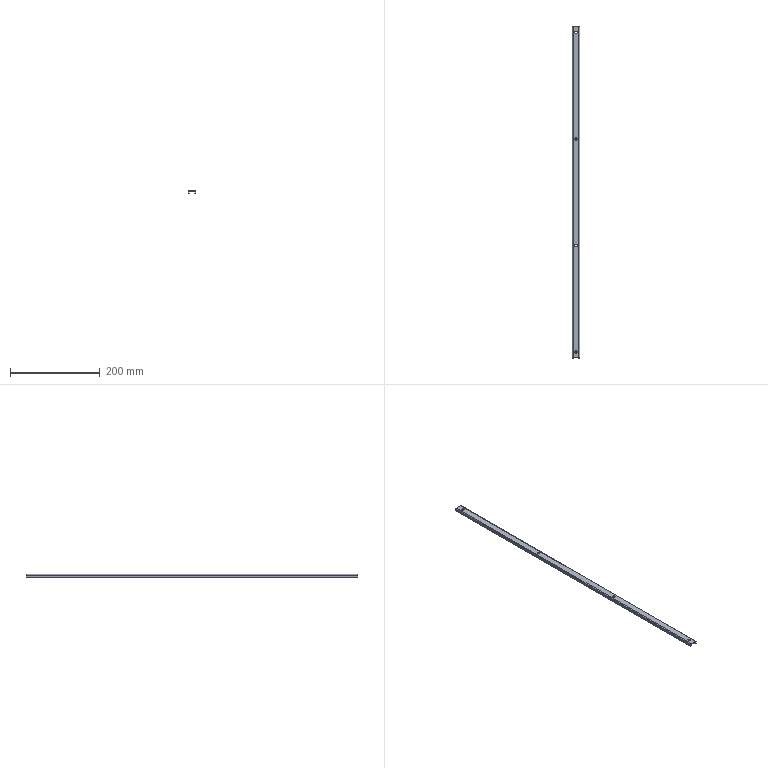Part | NX | features BREP 1 | 1 solid | 40 faces | box 17 x 738 x 7 mm | volume 38096 mm3 | plane 22 | cone 8 | cylinder 6 | torus 4 | commonest cylinder face diameters 0.2 x2 2 x2 4.2 x2
STEP:
#1=CARTESIAN_POINT('',(-2.7,355.,2.));
#2=VERTEX_POINT('',#1);
#3=CARTESIAN_POINT('',(2.7,355.,2.));
#4=VERTEX_POINT('',#3);
#5=CARTESIAN_POINT('',(0.,355.,2.));
#6=DIRECTION('',(0.,0.,1.));
#7=DIRECTION('',(1.,0.,0.));
#8=AXIS2_PLACEMENT_3D('',#5,#6,#7);
#9=CIRCLE('',#8,2.7);
#10=EDGE_CURVE('',#2,#4,#9,.T.);
#11=ORIENTED_EDGE('',*,*,#10,.T.);
#12=CARTESIAN_POINT('',(4.7,355.,0.));
#13=VERTEX_POINT('',#12);
#14=CARTESIAN_POINT('',(4.7,355.,0.));
#15=DIRECTION('',(0.7071,0.,-0.7071));
#16=VECTOR('',#15,1000.);
#17=LINE('',#14,#16);
#18=EDGE_CURVE('',#4,#13,#17,.T.);
#19=ORIENTED_EDGE('',*,*,#18,.T.);
#20=CARTESIAN_POINT('',(-4.7,355.,0.));
#21=VERTEX_POINT('',#20);
#22=CARTESIAN_POINT('',(0.,355.,0.));
#23=DIRECTION('',(0.,0.,-1.));
#24=DIRECTION('',(-1.,0.,0.));
#25=AXIS2_PLACEMENT_3D('',#22,#23,#24);
#26=CIRCLE('',#25,4.7);
#27=EDGE_CURVE('',#13,#21,#26,.T.);
#28=ORIENTED_EDGE('',*,*,#27,.T.);
#29=CARTESIAN_POINT('',(-4.7,355.,0.));
#30=DIRECTION('',(-0.7071,0.,-0.7071));
#31=VECTOR('',#30,1000.);
#32=LINE('',#29,#31);
#33=EDGE_CURVE('',#2,#21,#32,.T.);
#34=ORIENTED_EDGE('',*,*,#33,.F.);
#35=EDGE_LOOP('',(#11,#19,#28,#34));
#36=FACE_BOUND('',#35,.T.);
#37=CARTESIAN_POINT('',(0.,355.,0.));
#38=DIRECTION('',(0.,0.,-1.));
#39=DIRECTION('',(-1.,0.,0.));
#40=AXIS2_PLACEMENT_3D('',#37,#38,#39);
#41=CONICAL_SURFACE('',#40,4.7,0.7854);
#42=ADVANCED_FACE('',(#36),#41,.F.);
#43=CARTESIAN_POINT('',(-2.7,118.,2.));
#44=VERTEX_POINT('',#43);
#45=CARTESIAN_POINT('',(2.7,118.,2.));
#46=VERTEX_POINT('',#45);
#47=CARTESIAN_POINT('',(0.,118.,2.));
#48=DIRECTION('',(0.,0.,1.));
#49=DIRECTION('',(1.,0.,0.));
#50=AXIS2_PLACEMENT_3D('',#47,#48,#49);
#51=CIRCLE('',#50,2.7);
#52=EDGE_CURVE('',#44,#46,#51,.T.);
#53=ORIENTED_EDGE('',*,*,#52,.T.);
#54=CARTESIAN_POINT('',(4.7,118.,0.));
#55=VERTEX_POINT('',#54);
#56=CARTESIAN_POINT('',(4.7,118.,0.));
#57=DIRECTION('',(0.7071,0.,-0.7071));
#58=VECTOR('',#57,1000.);
#59=LINE('',#56,#58);
#60=EDGE_CURVE('',#46,#55,#59,.T.);
#61=ORIENTED_EDGE('',*,*,#60,.T.);
#62=CARTESIAN_POINT('',(-4.7,118.,0.));
#63=VERTEX_POINT('',#62);
#64=CARTESIAN_POINT('',(0.,118.,0.));
#65=DIRECTION('',(0.,0.,-1.));
#66=DIRECTION('',(-1.,0.,0.));
#67=AXIS2_PLACEMENT_3D('',#64,#65,#66);
#68=CIRCLE('',#67,4.7);
#69=EDGE_CURVE('',#55,#63,#68,.T.);
#70=ORIENTED_EDGE('',*,*,#69,.T.);
#71=CARTESIAN_POINT('',(-4.7,118.,0.));
#72=DIRECTION('',(-0.7071,0.,-0.7071));
#73=VECTOR('',#72,1000.);
#74=LINE('',#71,#73);
#75=EDGE_CURVE('',#44,#63,#74,.T.);
#76=ORIENTED_EDGE('',*,*,#75,.F.);
#77=EDGE_LOOP('',(#53,#61,#70,#76));
#78=FACE_BOUND('',#77,.T.);
#79=CARTESIAN_POINT('',(0.,118.,0.));
#80=DIRECTION('',(0.,0.,-1.));
#81=DIRECTION('',(-1.,0.,0.));
#82=AXIS2_PLACEMENT_3D('',#79,#80,#81);
#83=CONICAL_SURFACE('',#82,4.7,0.7854);
#84=ADVANCED_FACE('',(#78),#83,.F.);
#85=CARTESIAN_POINT('',(-2.7,-119.,2.));
#86=VERTEX_POINT('',#85);
#87=CARTESIAN_POINT('',(2.7,-119.,2.));
#88=VERTEX_POINT('',#87);
#89=CARTESIAN_POINT('',(0.,-119.,2.));
#90=DIRECTION('',(0.,0.,1.));
#91=DIRECTION('',(1.,0.,0.));
#92=AXIS2_PLACEMENT_3D('',#89,#90,#91);
#93=CIRCLE('',#92,2.7);
#94=EDGE_CURVE('',#86,#88,#93,.T.);
#95=ORIENTED_EDGE('',*,*,#94,.T.);
#96=CARTESIAN_POINT('',(4.7,-119.,0.));
#97=VERTEX_POINT('',#96);
#98=CARTESIAN_POINT('',(4.7,-119.,0.));
#99=DIRECTION('',(0.7071,0.,-0.7071));
#100=VECTOR('',#99,1000.);
#101=LINE('',#98,#100);
#102=EDGE_CURVE('',#88,#97,#101,.T.);
#103=ORIENTED_EDGE('',*,*,#102,.T.);
#104=CARTESIAN_POINT('',(-4.7,-119.,0.));
#105=VERTEX_POINT('',#104);
#106=CARTESIAN_POINT('',(0.,-119.,0.));
#107=DIRECTION('',(0.,0.,-1.));
#108=DIRECTION('',(-1.,0.,0.));
#109=AXIS2_PLACEMENT_3D('',#106,#107,#108);
#110=CIRCLE('',#109,4.7);
#111=EDGE_CURVE('',#97,#105,#110,.T.);
#112=ORIENTED_EDGE('',*,*,#111,.T.);
#113=CARTESIAN_POINT('',(-4.7,-119.,0.));
#114=DIRECTION('',(-0.7071,0.,-0.7071));
#115=VECTOR('',#114,1000.);
#116=LINE('',#113,#115);
#117=EDGE_CURVE('',#86,#105,#116,.T.);
#118=ORIENTED_EDGE('',*,*,#117,.F.);
#119=EDGE_LOOP('',(#95,#103,#112,#118));
#120=FACE_BOUND('',#119,.T.);
#121=CARTESIAN_POINT('',(0.,-119.,0.));
#122=DIRECTION('',(0.,0.,-1.));
#123=DIRECTION('',(-1.,0.,0.));
#124=AXIS2_PLACEMENT_3D('',#121,#122,#123);
#125=CONICAL_SURFACE('',#124,4.7,0.7854);
#126=ADVANCED_FACE('',(#120),#125,.F.);
#127=CARTESIAN_POINT('',(-2.7,-356.,2.));
#128=VERTEX_POINT('',#127);
#129=CARTESIAN_POINT('',(2.7,-356.,2.));
#130=VERTEX_POINT('',#129);
#131=CARTESIAN_POINT('',(0.,-356.,2.));
#132=DIRECTION('',(0.,0.,1.));
#133=DIRECTION('',(1.,0.,0.));
#134=AXIS2_PLACEMENT_3D('',#131,#132,#133);
#135=CIRCLE('',#134,2.7);
#136=EDGE_CURVE('',#128,#130,#135,.T.);
#137=ORIENTED_EDGE('',*,*,#136,.T.);
#138=CARTESIAN_POINT('',(4.7,-356.,0.));
#139=VERTEX_POINT('',#138);
#140=CARTESIAN_POINT('',(4.7,-356.,0.));
#141=DIRECTION('',(0.7071,0.,-0.7071));
#142=VECTOR('',#141,1000.);
#143=LINE('',#140,#142);
#144=EDGE_CURVE('',#130,#139,#143,.T.);
#145=ORIENTED_EDGE('',*,*,#144,.T.);
#146=CARTESIAN_POINT('',(-4.7,-356.,0.));
#147=VERTEX_POINT('',#146);
#148=CARTESIAN_POINT('',(0.,-356.,0.));
#149=DIRECTION('',(0.,0.,-1.));
#150=DIRECTION('',(-1.,0.,0.));
#151=AXIS2_PLACEMENT_3D('',#148,#149,#150);
#152=CIRCLE('',#151,4.7);
#153=EDGE_CURVE('',#139,#147,#152,.T.);
#154=ORIENTED_EDGE('',*,*,#153,.T.);
#155=CARTESIAN_POINT('',(-4.7,-356.,0.));
#156=DIRECTION('',(-0.7071,0.,-0.7071));
#157=VECTOR('',#156,1000.);
#158=LINE('',#155,#157);
#159=EDGE_CURVE('',#128,#147,#158,.T.);
#160=ORIENTED_EDGE('',*,*,#159,.F.);
#161=EDGE_LOOP('',(#137,#145,#154,#160));
#162=FACE_BOUND('',#161,.T.);
#163=CARTESIAN_POINT('',(0.,-356.,0.));
#164=DIRECTION('',(0.,0.,-1.));
#165=DIRECTION('',(-1.,0.,0.));
#166=AXIS2_PLACEMENT_3D('',#163,#164,#165);
#167=CONICAL_SURFACE('',#166,4.7,0.7854);
#168=ADVANCED_FACE('',(#162),#167,.F.);
#169=CARTESIAN_POINT('',(-6.4,368.,0.));
#170=VERTEX_POINT('',#169);
#171=CARTESIAN_POINT('',(-6.4,-368.,0.));
#172=VERTEX_POINT('',#171);
#173=CARTESIAN_POINT('',(-6.4,369.,0.));
#174=DIRECTION('',(0.,-1.,0.));
#175=VECTOR('',#174,1000.);
#176=LINE('',#173,#175);
#177=EDGE_CURVE('',#170,#172,#176,.T.);
#178=ORIENTED_EDGE('',*,*,#177,.F.);
#179=CARTESIAN_POINT('',(6.4,368.,0.));
#180=VERTEX_POINT('',#179);
#181=CARTESIAN_POINT('',(6.4,368.,0.));
#182=DIRECTION('',(1.,0.,0.));
#183=VECTOR('',#182,1000.);
#184=LINE('',#181,#183);
#185=EDGE_CURVE('',#170,#180,#184,.T.);
#186=ORIENTED_EDGE('',*,*,#185,.T.);
#187=CARTESIAN_POINT('',(6.4,-368.,0.));
#188=VERTEX_POINT('',#187);
#189=CARTESIAN_POINT('',(6.4,369.,0.));
#190=DIRECTION('',(0.,-1.,0.));
#191=VECTOR('',#190,1000.);
#192=LINE('',#189,#191);
#193=EDGE_CURVE('',#180,#188,#192,.T.);
#194=ORIENTED_EDGE('',*,*,#193,.T.);
#195=CARTESIAN_POINT('',(-6.4,-368.,0.));
#196=DIRECTION('',(-1.,0.,0.));
#197=VECTOR('',#196,1000.);
#198=LINE('',#195,#197);
#199=EDGE_CURVE('',#188,#172,#198,.T.);
#200=ORIENTED_EDGE('',*,*,#199,.T.);
#201=EDGE_LOOP('',(#178,#186,#194,#200));
#202=FACE_BOUND('',#201,.T.);
#203=CARTESIAN_POINT('',(0.,355.,0.));
#204=DIRECTION('',(0.,0.,-1.));
#205=DIRECTION('',(-1.,0.,0.));
#206=AXIS2_PLACEMENT_3D('',#203,#204,#205);
#207=CIRCLE('',#206,4.7);
#208=EDGE_CURVE('',#21,#13,#207,.T.);
#209=ORIENTED_EDGE('',*,*,#208,.F.);
#210=ORIENTED_EDGE('',*,*,#27,.F.);
#211=EDGE_LOOP('',(#209,#210));
#212=FACE_BOUND('',#211,.T.);
#213=CARTESIAN_POINT('',(0.,118.,0.));
#214=DIRECTION('',(0.,0.,-1.));
#215=DIRECTION('',(-1.,0.,0.));
#216=AXIS2_PLACEMENT_3D('',#213,#214,#215);
#217=CIRCLE('',#216,4.7);
#218=EDGE_CURVE('',#63,#55,#217,.T.);
#219=ORIENTED_EDGE('',*,*,#218,.F.);
#220=ORIENTED_EDGE('',*,*,#69,.F.);
#221=EDGE_LOOP('',(#219,#220));
#222=FACE_BOUND('',#221,.T.);
#223=CARTESIAN_POINT('',(0.,-356.,0.));
#224=DIRECTION('',(0.,0.,-1.));
#225=DIRECTION('',(-1.,0.,0.));
#226=AXIS2_PLACEMENT_3D('',#223,#224,#225);
#227=CIRCLE('',#226,4.7);
#228=EDGE_CURVE('',#147,#139,#227,.T.);
#229=ORIENTED_EDGE('',*,*,#228,.F.);
#230=ORIENTED_EDGE('',*,*,#153,.F.);
#231=EDGE_LOOP('',(#229,#230));
#232=FACE_BOUND('',#231,.T.);
#233=CARTESIAN_POINT('',(0.,-119.,0.));
#234=DIRECTION('',(0.,0.,-1.));
#235=DIRECTION('',(-1.,0.,0.));
#236=AXIS2_PLACEMENT_3D('',#233,#234,#235);
#237=CIRCLE('',#236,4.7);
#238=EDGE_CURVE('',#105,#97,#237,.T.);
#239=ORIENTED_EDGE('',*,*,#238,.F.);
#240=ORIENTED_EDGE('',*,*,#111,.F.);
#241=EDGE_LOOP('',(#239,#240));
#242=FACE_BOUND('',#241,.T.);
#243=CARTESIAN_POINT('',(-6.5,369.,0.));
#244=DIRECTION('',(0.,0.,1.));
#245=DIRECTION('',(1.,0.,0.));
#246=AXIS2_PLACEMENT_3D('',#243,#244,#245);
#247=PLANE('',#246);
#248=ADVANCED_FACE('',(#202,#212,#222,#232,#242),#247,.F.);
#249=CARTESIAN_POINT('',(6.4,-369.,2.));
#250=VERTEX_POINT('',#249);
#251=CARTESIAN_POINT('',(-6.4,-369.,2.));
#252=VERTEX_POINT('',#251);
#253=CARTESIAN_POINT('',(-6.5,-369.,2.));
#254=DIRECTION('',(-1.,0.,0.));
#255=VECTOR('',#254,1000.);
#256=LINE('',#253,#255);
#257=EDGE_CURVE('',#250,#252,#256,.T.);
#258=ORIENTED_EDGE('',*,*,#257,.F.);
#259=CARTESIAN_POINT('',(6.4,369.,2.));
#260=VERTEX_POINT('',#259);
#261=CARTESIAN_POINT('',(6.4,369.,2.));
#262=DIRECTION('',(0.,-1.,0.));
#263=VECTOR('',#262,1000.);
#264=LINE('',#261,#263);
#265=EDGE_CURVE('',#260,#250,#264,.T.);
#266=ORIENTED_EDGE('',*,*,#265,.F.);
#267=CARTESIAN_POINT('',(-6.4,369.,2.));
#268=VERTEX_POINT('',#267);
#269=CARTESIAN_POINT('',(-6.5,369.,2.));
#270=DIRECTION('',(-1.,0.,0.));
#271=VECTOR('',#270,1000.);
#272=LINE('',#269,#271);
#273=EDGE_CURVE('',#260,#268,#272,.T.);
#274=ORIENTED_EDGE('',*,*,#273,.T.);
#275=CARTESIAN_POINT('',(-6.4,369.,2.));
#276=DIRECTION('',(0.,-1.,0.));
#277=VECTOR('',#276,1000.);
#278=LINE('',#275,#277);
#279=EDGE_CURVE('',#268,#252,#278,.T.);
#280=ORIENTED_EDGE('',*,*,#279,.T.);
#281=EDGE_LOOP('',(#258,#266,#274,#280));
#282=FACE_BOUND('',#281,.T.);
#283=ORIENTED_EDGE('',*,*,#10,.F.);
#284=CARTESIAN_POINT('',(0.,355.,2.));
#285=DIRECTION('',(0.,0.,1.));
#286=DIRECTION('',(1.,0.,0.));
#287=AXIS2_PLACEMENT_3D('',#284,#285,#286);
#288=CIRCLE('',#287,2.7);
#289=EDGE_CURVE('',#4,#2,#288,.T.);
#290=ORIENTED_EDGE('',*,*,#289,.F.);
#291=EDGE_LOOP('',(#283,#290));
#292=FACE_BOUND('',#291,.T.);
#293=ORIENTED_EDGE('',*,*,#52,.F.);
#294=CARTESIAN_POINT('',(0.,118.,2.));
#295=DIRECTION('',(0.,0.,1.));
#296=DIRECTION('',(1.,0.,0.));
#297=AXIS2_PLACEMENT_3D('',#294,#295,#296);
#298=CIRCLE('',#297,2.7);
#299=EDGE_CURVE('',#46,#44,#298,.T.);
#300=ORIENTED_EDGE('',*,*,#299,.F.);
#301=EDGE_LOOP('',(#293,#300));
#302=FACE_BOUND('',#301,.T.);
#303=ORIENTED_EDGE('',*,*,#94,.F.);
#304=CARTESIAN_POINT('',(0.,-119.,2.));
#305=DIRECTION('',(0.,0.,1.));
#306=DIRECTION('',(1.,0.,0.));
#307=AXIS2_PLACEMENT_3D('',#304,#305,#306);
#308=CIRCLE('',#307,2.7);
#309=EDGE_CURVE('',#88,#86,#308,.T.);
#310=ORIENTED_EDGE('',*,*,#309,.F.);
#311=EDGE_LOOP('',(#303,#310));
#312=FACE_BOUND('',#311,.T.);
#313=ORIENTED_EDGE('',*,*,#136,.F.);
#314=CARTESIAN_POINT('',(0.,-356.,2.));
#315=DIRECTION('',(0.,0.,1.));
#316=DIRECTION('',(1.,0.,0.));
#317=AXIS2_PLACEMENT_3D('',#314,#315,#316);
#318=CIRCLE('',#317,2.7);
#319=EDGE_CURVE('',#130,#128,#318,.T.);
#320=ORIENTED_EDGE('',*,*,#319,.F.);
#321=EDGE_LOOP('',(#313,#320));
#322=FACE_BOUND('',#321,.T.);
#323=CARTESIAN_POINT('',(-6.5,369.,2.));
#324=DIRECTION('',(0.,0.,1.));
#325=DIRECTION('',(1.,0.,0.));
#326=AXIS2_PLACEMENT_3D('',#323,#324,#325);
#327=PLANE('',#326);
#328=ADVANCED_FACE('',(#282,#292,#302,#312,#322),#327,.T.);
#329=CARTESIAN_POINT('',(7.5,369.,-0.1));
#330=VERTEX_POINT('',#329);
#331=CARTESIAN_POINT('',(8.5,369.,-0.1));
#332=VERTEX_POINT('',#331);
#333=CARTESIAN_POINT('',(6.5,369.,-0.1));
#334=DIRECTION('',(1.,0.,0.));
#335=VECTOR('',#334,1000.);
#336=LINE('',#333,#335);
#337=EDGE_CURVE('',#330,#332,#336,.T.);
#338=ORIENTED_EDGE('',*,*,#337,.F.);
#339=CARTESIAN_POINT('',(6.4,369.,1.));
#340=VERTEX_POINT('',#339);
#341=CARTESIAN_POINT('',(6.4,369.,-0.1));
#342=DIRECTION('',(0.,-1.,0.));
#343=DIRECTION('',(0.,0.,1.));
#344=AXIS2_PLACEMENT_3D('',#341,#342,#343);
#345=CIRCLE('',#344,1.1);
#346=EDGE_CURVE('',#330,#340,#345,.T.);
#347=ORIENTED_EDGE('',*,*,#346,.T.);
#348=CARTESIAN_POINT('',(6.4,369.,2.));
#349=DIRECTION('',(0.,0.,-1.));
#350=VECTOR('',#349,1000.);
#351=LINE('',#348,#350);
#352=EDGE_CURVE('',#260,#340,#351,.T.);
#353=ORIENTED_EDGE('',*,*,#352,.F.);
#354=CARTESIAN_POINT('',(6.4,369.,-0.1));
#355=DIRECTION('',(0.,-1.,0.));
#356=DIRECTION('',(1.,0.,0.));
#357=AXIS2_PLACEMENT_3D('',#354,#355,#356);
#358=CIRCLE('',#357,2.1);
#359=EDGE_CURVE('',#332,#260,#358,.T.);
#360=ORIENTED_EDGE('',*,*,#359,.F.);
#361=EDGE_LOOP('',(#338,#347,#353,#360));
#362=FACE_BOUND('',#361,.T.);
#363=CARTESIAN_POINT('',(6.5,369.,-0.1));
#364=DIRECTION('',(0.,1.,0.));
#365=DIRECTION('',(1.,0.,0.));
#366=AXIS2_PLACEMENT_3D('',#363,#364,#365);
#367=PLANE('',#366);
#368=ADVANCED_FACE('',(#362),#367,.T.);
#369=CARTESIAN_POINT('',(8.5,369.,-4.));
#370=VERTEX_POINT('',#369);
#371=CARTESIAN_POINT('',(8.5,369.,0.));
#372=DIRECTION('',(0.,0.,1.));
#373=VECTOR('',#372,1000.);
#374=LINE('',#371,#373);
#375=EDGE_CURVE('',#370,#332,#374,.T.);
#376=ORIENTED_EDGE('',*,*,#375,.F.);
#377=CARTESIAN_POINT('',(6.5,369.,-4.));
#378=VERTEX_POINT('',#377);
#379=CARTESIAN_POINT('',(6.4,369.,-4.));
#380=DIRECTION('',(-1.,0.,0.));
#381=VECTOR('',#380,1000.);
#382=LINE('',#379,#381);
#383=EDGE_CURVE('',#370,#378,#382,.T.);
#384=ORIENTED_EDGE('',*,*,#383,.T.);
#385=CARTESIAN_POINT('',(6.5,369.,-1.195));
#386=VERTEX_POINT('',#385);
#387=CARTESIAN_POINT('',(6.5,369.,0.));
#388=DIRECTION('',(0.,0.,1.));
#389=VECTOR('',#388,1000.);
#390=LINE('',#387,#389);
#391=EDGE_CURVE('',#378,#386,#390,.T.);
#392=ORIENTED_EDGE('',*,*,#391,.T.);
#393=CARTESIAN_POINT('',(6.4,369.,-0.1));
#394=DIRECTION('',(0.,-1.,0.));
#395=DIRECTION('',(0.,0.,1.));
#396=AXIS2_PLACEMENT_3D('',#393,#394,#395);
#397=CIRCLE('',#396,1.1);
#398=EDGE_CURVE('',#386,#330,#397,.T.);
#399=ORIENTED_EDGE('',*,*,#398,.T.);
#400=ORIENTED_EDGE('',*,*,#337,.T.);
#401=EDGE_LOOP('',(#376,#384,#392,#399,#400));
#402=FACE_BOUND('',#401,.T.);
#403=CARTESIAN_POINT('',(6.4,369.,2.));
#404=DIRECTION('',(0.,1.,0.));
#405=DIRECTION('',(1.,0.,0.));
#406=AXIS2_PLACEMENT_3D('',#403,#404,#405);
#407=PLANE('',#406);
#408=ADVANCED_FACE('',(#402),#407,.T.);
#409=CARTESIAN_POINT('',(6.4,-369.,1.));
#410=VERTEX_POINT('',#409);
#411=CARTESIAN_POINT('',(6.4,-369.,0.));
#412=DIRECTION('',(0.,0.,1.));
#413=VECTOR('',#412,1000.);
#414=LINE('',#411,#413);
#415=EDGE_CURVE('',#410,#250,#414,.T.);
#416=ORIENTED_EDGE('',*,*,#415,.F.);
#417=CARTESIAN_POINT('',(7.5,-369.,-0.1));
#418=VERTEX_POINT('',#417);
#419=CARTESIAN_POINT('',(6.4,-369.,-0.1));
#420=DIRECTION('',(0.,1.,0.));
#421=DIRECTION('',(0.,0.,-1.));
#422=AXIS2_PLACEMENT_3D('',#419,#420,#421);
#423=CIRCLE('',#422,1.1);
#424=EDGE_CURVE('',#410,#418,#423,.T.);
#425=ORIENTED_EDGE('',*,*,#424,.T.);
#426=CARTESIAN_POINT('',(8.5,-369.,-0.1));
#427=VERTEX_POINT('',#426);
#428=CARTESIAN_POINT('',(8.5,-369.,-0.1));
#429=DIRECTION('',(-1.,0.,0.));
#430=VECTOR('',#429,1000.);
#431=LINE('',#428,#430);
#432=EDGE_CURVE('',#427,#418,#431,.T.);
#433=ORIENTED_EDGE('',*,*,#432,.F.);
#434=CARTESIAN_POINT('',(6.4,-369.,-0.1));
#435=DIRECTION('',(0.,-1.,0.));
#436=DIRECTION('',(1.,0.,0.));
#437=AXIS2_PLACEMENT_3D('',#434,#435,#436);
#438=CIRCLE('',#437,2.1);
#439=EDGE_CURVE('',#427,#250,#438,.T.);
#440=ORIENTED_EDGE('',*,*,#439,.T.);
#441=EDGE_LOOP('',(#416,#425,#433,#440));
#442=FACE_BOUND('',#441,.T.);
#443=CARTESIAN_POINT('',(6.4,-369.,0.));
#444=DIRECTION('',(0.,-1.,0.));
#445=DIRECTION('',(0.,0.,-1.));
#446=AXIS2_PLACEMENT_3D('',#443,#444,#445);
#447=PLANE('',#446);
#448=ADVANCED_FACE('',(#442),#447,.T.);
#449=CARTESIAN_POINT('',(-6.4,-369.,1.));
#450=VERTEX_POINT('',#449);
#451=CARTESIAN_POINT('',(-6.4,-369.,2.));
#452=DIRECTION('',(0.,0.,-1.));
#453=VECTOR('',#452,1000.);
#454=LINE('',#451,#453);
#455=EDGE_CURVE('',#252,#450,#454,.T.);
#456=ORIENTED_EDGE('',*,*,#455,.T.);
#457=CARTESIAN_POINT('',(6.4,-369.,1.));
#458=DIRECTION('',(1.,0.,0.));
#459=VECTOR('',#458,1000.);
#460=LINE('',#457,#459);
#461=EDGE_CURVE('',#450,#410,#460,.T.);
#462=ORIENTED_EDGE('',*,*,#461,.T.);
#463=ORIENTED_EDGE('',*,*,#415,.T.);
#464=ORIENTED_EDGE('',*,*,#257,.T.);
#465=EDGE_LOOP('',(#456,#462,#463,#464));
#466=FACE_BOUND('',#465,.T.);
#467=CARTESIAN_POINT('',(8.5,-369.,-0.1));
#468=DIRECTION('',(0.,-1.,0.));
#469=DIRECTION('',(0.,0.,-1.));
#470=AXIS2_PLACEMENT_3D('',#467,#468,#469);
#471=PLANE('',#470);
#472=ADVANCED_FACE('',(#466),#471,.T.);
#473=CARTESIAN_POINT('',(-6.4,369.,1.));
#474=VERTEX_POINT('',#473);
#475=CARTESIAN_POINT('',(-6.4,369.,0.));
#476=DIRECTION('',(0.,0.,1.));
#477=VECTOR('',#476,1000.);
#478=LINE('',#475,#477);
#479=EDGE_CURVE('',#474,#268,#478,.T.);
#480=ORIENTED_EDGE('',*,*,#479,.F.);
#481=CARTESIAN_POINT('',(-7.5,369.,-0.1));
#482=VERTEX_POINT('',#481);
#483=CARTESIAN_POINT('',(-6.4,369.,-0.1));
#484=DIRECTION('',(0.,-1.,0.));
#485=DIRECTION('',(0.,0.,1.));
#486=AXIS2_PLACEMENT_3D('',#483,#484,#485);
#487=CIRCLE('',#486,1.1);
#488=EDGE_CURVE('',#474,#482,#487,.T.);
#489=ORIENTED_EDGE('',*,*,#488,.T.);
#490=CARTESIAN_POINT('',(-8.5,369.,-0.1));
#491=VERTEX_POINT('',#490);
#492=CARTESIAN_POINT('',(-8.5,369.,-0.1));
#493=DIRECTION('',(1.,0.,0.));
#494=VECTOR('',#493,1000.);
#495=LINE('',#492,#494);
#496=EDGE_CURVE('',#491,#482,#495,.T.);
#497=ORIENTED_EDGE('',*,*,#496,.F.);
#498=CARTESIAN_POINT('',(-6.4,369.,-0.1));
#499=DIRECTION('',(0.,-1.,0.));
#500=DIRECTION('',(1.,0.,0.));
#501=AXIS2_PLACEMENT_3D('',#498,#499,#500);
#502=CIRCLE('',#501,2.1);
#503=EDGE_CURVE('',#268,#491,#502,.T.);
#504=ORIENTED_EDGE('',*,*,#503,.F.);
#505=EDGE_LOOP('',(#480,#489,#497,#504));
#506=FACE_BOUND('',#505,.T.);
#507=CARTESIAN_POINT('',(-6.4,369.,0.));
#508=DIRECTION('',(0.,1.,0.));
#509=DIRECTION('',(1.,0.,0.));
#510=AXIS2_PLACEMENT_3D('',#507,#508,#509);
#511=PLANE('',#510);
#512=ADVANCED_FACE('',(#506),#511,.T.);
#513=ORIENTED_EDGE('',*,*,#352,.T.);
#514=CARTESIAN_POINT('',(-6.4,369.,1.));
#515=DIRECTION('',(-1.,0.,0.));
#516=VECTOR('',#515,1000.);
#517=LINE('',#514,#516);
#518=EDGE_CURVE('',#340,#474,#517,.T.);
#519=ORIENTED_EDGE('',*,*,#518,.T.);
#520=ORIENTED_EDGE('',*,*,#479,.T.);
#521=ORIENTED_EDGE('',*,*,#273,.F.);
#522=EDGE_LOOP('',(#513,#519,#520,#521));
#523=FACE_BOUND('',#522,.T.);
#524=CARTESIAN_POINT('',(-8.5,369.,-0.1));
#525=DIRECTION('',(0.,1.,0.));
#526=DIRECTION('',(1.,0.,0.));
#527=AXIS2_PLACEMENT_3D('',#524,#525,#526);
#528=PLANE('',#527);
#529=ADVANCED_FACE('',(#523),#528,.T.);
#530=CARTESIAN_POINT('',(-7.5,-369.,-0.1));
#531=VERTEX_POINT('',#530);
#532=CARTESIAN_POINT('',(-8.5,-369.,-0.1));
#533=VERTEX_POINT('',#532);
#534=CARTESIAN_POINT('',(-6.5,-369.,-0.1));
#535=DIRECTION('',(-1.,0.,0.));
#536=VECTOR('',#535,1000.);
#537=LINE('',#534,#536);
#538=EDGE_CURVE('',#531,#533,#537,.T.);
#539=ORIENTED_EDGE('',*,*,#538,.F.);
#540=CARTESIAN_POINT('',(-6.4,-369.,-0.1));
#541=DIRECTION('',(0.,1.,0.));
#542=DIRECTION('',(0.,0.,-1.));
#543=AXIS2_PLACEMENT_3D('',#540,#541,#542);
#544=CIRCLE('',#543,1.1);
#545=EDGE_CURVE('',#531,#450,#544,.T.);
#546=ORIENTED_EDGE('',*,*,#545,.T.);
#547=ORIENTED_EDGE('',*,*,#455,.F.);
#548=CARTESIAN_POINT('',(-6.4,-369.,-0.1));
#549=DIRECTION('',(0.,-1.,0.));
#550=DIRECTION('',(1.,0.,0.));
#551=AXIS2_PLACEMENT_3D('',#548,#549,#550);
#552=CIRCLE('',#551,2.1);
#553=EDGE_CURVE('',#252,#533,#552,.T.);
#554=ORIENTED_EDGE('',*,*,#553,.T.);
#555=EDGE_LOOP('',(#539,#546,#547,#554));
#556=FACE_BOUND('',#555,.T.);
#557=CARTESIAN_POINT('',(-6.5,-369.,-0.1));
#558=DIRECTION('',(0.,-1.,0.));
#559=DIRECTION('',(0.,0.,-1.));
#560=AXIS2_PLACEMENT_3D('',#557,#558,#559);
#561=PLANE('',#560);
#562=ADVANCED_FACE('',(#556),#561,.T.);
#563=CARTESIAN_POINT('',(-8.5,-369.,-4.));
#564=VERTEX_POINT('',#563);
#565=CARTESIAN_POINT('',(-8.5,-369.,0.));
#566=DIRECTION('',(0.,0.,-1.));
#567=VECTOR('',#566,1000.);
#568=LINE('',#565,#567);
#569=EDGE_CURVE('',#533,#564,#568,.T.);
#570=ORIENTED_EDGE('',*,*,#569,.T.);
#571=CARTESIAN_POINT('',(-6.5,-369.,-4.));
#572=VERTEX_POINT('',#571);
#573=CARTESIAN_POINT('',(-6.4,-369.,-4.));
#574=DIRECTION('',(1.,0.,0.));
#575=VECTOR('',#574,1000.);
#576=LINE('',#573,#575);
#577=EDGE_CURVE('',#564,#572,#576,.T.);
#578=ORIENTED_EDGE('',*,*,#577,.T.);
#579=CARTESIAN_POINT('',(-6.5,-369.,-1.195));
#580=VERTEX_POINT('',#579);
#581=CARTESIAN_POINT('',(-6.5,-369.,0.));
#582=DIRECTION('',(0.,0.,-1.));
#583=VECTOR('',#582,1000.);
#584=LINE('',#581,#583);
#585=EDGE_CURVE('',#580,#572,#584,.T.);
#586=ORIENTED_EDGE('',*,*,#585,.F.);
#587=CARTESIAN_POINT('',(-6.4,-369.,-0.1));
#588=DIRECTION('',(0.,1.,0.));
#589=DIRECTION('',(0.,0.,-1.));
#590=AXIS2_PLACEMENT_3D('',#587,#588,#589);
#591=CIRCLE('',#590,1.1);
#592=EDGE_CURVE('',#580,#531,#591,.T.);
#593=ORIENTED_EDGE('',*,*,#592,.T.);
#594=ORIENTED_EDGE('',*,*,#538,.T.);
#595=EDGE_LOOP('',(#570,#578,#586,#593,#594));
#596=FACE_BOUND('',#595,.T.);
#597=CARTESIAN_POINT('',(-6.4,-369.,2.));
#598=DIRECTION('',(0.,-1.,0.));
#599=DIRECTION('',(0.,0.,-1.));
#600=AXIS2_PLACEMENT_3D('',#597,#598,#599);
#601=PLANE('',#600);
#602=ADVANCED_FACE('',(#596),#601,.T.);
#603=CARTESIAN_POINT('',(-6.5,368.,-5.));
#604=VERTEX_POINT('',#603);
#605=CARTESIAN_POINT('',(-6.5,-368.,-5.));
#606=VERTEX_POINT('',#605);
#607=CARTESIAN_POINT('',(-6.5,369.,-5.));
#608=DIRECTION('',(0.,-1.,0.));
#609=VECTOR('',#608,1000.);
#610=LINE('',#607,#609);
#611=EDGE_CURVE('',#604,#606,#610,.T.);
#612=ORIENTED_EDGE('',*,*,#611,.F.);
#613=CARTESIAN_POINT('',(-6.5,369.,-4.));
#614=VERTEX_POINT('',#613);
#615=CARTESIAN_POINT('',(-6.5,368.,-5.));
#616=DIRECTION('',(0.,0.7071,0.7071));
#617=VECTOR('',#616,1000.);
#618=LINE('',#615,#617);
#619=EDGE_CURVE('',#604,#614,#618,.T.);
#620=ORIENTED_EDGE('',*,*,#619,.T.);
#621=CARTESIAN_POINT('',(-6.5,369.,-1.195));
#622=VERTEX_POINT('',#621);
#623=CARTESIAN_POINT('',(-6.5,369.,0.));
#624=DIRECTION('',(0.,0.,-1.));
#625=VECTOR('',#624,1000.);
#626=LINE('',#623,#625);
#627=EDGE_CURVE('',#622,#614,#626,.T.);
#628=ORIENTED_EDGE('',*,*,#627,.F.);
#629=CARTESIAN_POINT('',(-6.5,368.,-0.1));
#630=VERTEX_POINT('',#629);
#631=CARTESIAN_POINT('',(-6.5,369.,-1.195));
#632=CARTESIAN_POINT('',(-6.5,369.,-0.9262));
#633=CARTESIAN_POINT('',(-6.5,368.841,-0.5362));
#634=CARTESIAN_POINT('',(-6.5,368.369,-0.219));
#635=CARTESIAN_POINT('',(-6.5,368.163,-0.1517));
#636=CARTESIAN_POINT('',(-6.5,368.,-0.1));
#637=B_SPLINE_CURVE_WITH_KNOTS('',3,(#631,#632,#633,#634,#635,#636),.UNSPECIFIED.,.F.,.F.,(4,1,1,4),(0.,0.5,0.75,1.),.UNSPECIFIED.);
#638=EDGE_CURVE('',#622,#630,#637,.T.);
#639=ORIENTED_EDGE('',*,*,#638,.T.);
#640=CARTESIAN_POINT('',(-6.5,-368.,-0.1));
#641=VERTEX_POINT('',#640);
#642=CARTESIAN_POINT('',(-6.5,369.,-0.1));
#643=DIRECTION('',(0.,-1.,0.));
#644=VECTOR('',#643,1000.);
#645=LINE('',#642,#644);
#646=EDGE_CURVE('',#630,#641,#645,.T.);
#647=ORIENTED_EDGE('',*,*,#646,.T.);
#648=CARTESIAN_POINT('',(-6.5,-368.,-0.1));
#649=CARTESIAN_POINT('',(-6.5,-368.162,-0.1513));
#650=CARTESIAN_POINT('',(-6.5,-368.369,-0.2191));
#651=CARTESIAN_POINT('',(-6.5,-368.84,-0.5364));
#652=CARTESIAN_POINT('',(-6.5,-369.,-0.9248));
#653=CARTESIAN_POINT('',(-6.5,-369.,-1.195));
#654=B_SPLINE_CURVE_WITH_KNOTS('',3,(#648,#649,#650,#651,#652,#653),.UNSPECIFIED.,.F.,.F.,(4,1,1,4),(0.,0.25,0.5,1.),.UNSPECIFIED.);
#655=EDGE_CURVE('',#641,#580,#654,.T.);
#656=ORIENTED_EDGE('',*,*,#655,.T.);
#657=ORIENTED_EDGE('',*,*,#585,.T.);
#658=CARTESIAN_POINT('',(-6.5,-369.,-4.));
#659=DIRECTION('',(0.,0.7071,-0.7071));
#660=VECTOR('',#659,1000.);
#661=LINE('',#658,#660);
#662=EDGE_CURVE('',#572,#606,#661,.T.);
#663=ORIENTED_EDGE('',*,*,#662,.T.);
#664=EDGE_LOOP('',(#612,#620,#628,#639,#647,#656,#657,#663));
#665=FACE_BOUND('',#664,.T.);
#666=CARTESIAN_POINT('',(-6.5,369.,0.));
#667=DIRECTION('',(-1.,0.,0.));
#668=DIRECTION('',(0.,1.,0.));
#669=AXIS2_PLACEMENT_3D('',#666,#667,#668);
#670=PLANE('',#669);
#671=ADVANCED_FACE('',(#665),#670,.F.);
#672=CARTESIAN_POINT('',(-8.5,368.,-5.));
#673=VERTEX_POINT('',#672);
#674=CARTESIAN_POINT('',(-8.5,-368.,-5.));
#675=VERTEX_POINT('',#674);
#676=CARTESIAN_POINT('',(-8.5,369.,-5.));
#677=DIRECTION('',(0.,-1.,0.));
#678=VECTOR('',#677,1000.);
#679=LINE('',#676,#678);
#680=EDGE_CURVE('',#673,#675,#679,.T.);
#681=ORIENTED_EDGE('',*,*,#680,.F.);
#682=CARTESIAN_POINT('',(-8.5,368.,-5.));
#683=DIRECTION('',(1.,0.,0.));
#684=VECTOR('',#683,1000.);
#685=LINE('',#682,#684);
#686=EDGE_CURVE('',#673,#604,#685,.T.);
#687=ORIENTED_EDGE('',*,*,#686,.T.);
#688=ORIENTED_EDGE('',*,*,#611,.T.);
#689=CARTESIAN_POINT('',(-8.5,-368.,-5.));
#690=DIRECTION('',(-1.,0.,0.));
#691=VECTOR('',#690,1000.);
#692=LINE('',#689,#691);
#693=EDGE_CURVE('',#606,#675,#692,.T.);
#694=ORIENTED_EDGE('',*,*,#693,.T.);
#695=EDGE_LOOP('',(#681,#687,#688,#694));
#696=FACE_BOUND('',#695,.T.);
#697=CARTESIAN_POINT('',(-8.5,369.,-5.));
#698=DIRECTION('',(0.,0.,-1.));
#699=DIRECTION('',(-1.,0.,0.));
#700=AXIS2_PLACEMENT_3D('',#697,#698,#699);
#701=PLANE('',#700);
#702=ADVANCED_FACE('',(#696),#701,.T.);
#703=CARTESIAN_POINT('',(-8.5,369.,-4.));
#704=VERTEX_POINT('',#703);
#705=CARTESIAN_POINT('',(-8.5,369.,0.));
#706=DIRECTION('',(0.,0.,-1.));
#707=VECTOR('',#706,1000.);
#708=LINE('',#705,#707);
#709=EDGE_CURVE('',#491,#704,#708,.T.);
#710=ORIENTED_EDGE('',*,*,#709,.T.);
#711=CARTESIAN_POINT('',(-8.5,371.,-2.));
#712=DIRECTION('',(0.,-0.7071,-0.7071));
#713=VECTOR('',#712,1000.);
#714=LINE('',#711,#713);
#715=EDGE_CURVE('',#704,#673,#714,.T.);
#716=ORIENTED_EDGE('',*,*,#715,.T.);
#717=ORIENTED_EDGE('',*,*,#680,.T.);
#718=CARTESIAN_POINT('',(-8.5,-2.,-371.));
#719=DIRECTION('',(0.,-0.7071,0.7071));
#720=VECTOR('',#719,1000.);
#721=LINE('',#718,#720);
#722=EDGE_CURVE('',#675,#564,#721,.T.);
#723=ORIENTED_EDGE('',*,*,#722,.T.);
#724=ORIENTED_EDGE('',*,*,#569,.F.);
#725=CARTESIAN_POINT('',(-8.5,369.,-0.1));
#726=DIRECTION('',(0.,-1.,0.));
#727=VECTOR('',#726,1000.);
#728=LINE('',#725,#727);
#729=EDGE_CURVE('',#491,#533,#728,.T.);
#730=ORIENTED_EDGE('',*,*,#729,.F.);
#731=EDGE_LOOP('',(#710,#716,#717,#723,#724,#730));
#732=FACE_BOUND('',#731,.T.);
#733=CARTESIAN_POINT('',(-8.5,369.,0.));
#734=DIRECTION('',(-1.,0.,0.));
#735=DIRECTION('',(0.,1.,0.));
#736=AXIS2_PLACEMENT_3D('',#733,#734,#735);
#737=PLANE('',#736);
#738=ADVANCED_FACE('',(#732),#737,.T.);
#739=ORIENTED_EDGE('',*,*,#553,.F.);
#740=ORIENTED_EDGE('',*,*,#279,.F.);
#741=ORIENTED_EDGE('',*,*,#503,.T.);
#742=ORIENTED_EDGE('',*,*,#729,.T.);
#743=EDGE_LOOP('',(#739,#740,#741,#742));
#744=FACE_BOUND('',#743,.T.);
#745=CARTESIAN_POINT('',(-6.4,369.,-0.1));
#746=DIRECTION('',(0.,-1.,0.));
#747=DIRECTION('',(0.,0.,-1.));
#748=AXIS2_PLACEMENT_3D('',#745,#746,#747);
#749=CYLINDRICAL_SURFACE('',#748,2.1);
#750=ADVANCED_FACE('',(#744),#749,.T.);
#751=ORIENTED_EDGE('',*,*,#439,.F.);
#752=CARTESIAN_POINT('',(8.5,369.,-0.1));
#753=DIRECTION('',(0.,-1.,0.));
#754=VECTOR('',#753,1000.);
#755=LINE('',#752,#754);
#756=EDGE_CURVE('',#332,#427,#755,.T.);
#757=ORIENTED_EDGE('',*,*,#756,.F.);
#758=ORIENTED_EDGE('',*,*,#359,.T.);
#759=ORIENTED_EDGE('',*,*,#265,.T.);
#760=EDGE_LOOP('',(#751,#757,#758,#759));
#761=FACE_BOUND('',#760,.T.);
#762=CARTESIAN_POINT('',(6.4,369.,-0.1));
#763=DIRECTION('',(0.,-1.,0.));
#764=DIRECTION('',(0.,0.,-1.));
#765=AXIS2_PLACEMENT_3D('',#762,#763,#764);
#766=CYLINDRICAL_SURFACE('',#765,2.1);
#767=ADVANCED_FACE('',(#761),#766,.T.);
#768=CARTESIAN_POINT('',(8.5,368.,-5.));
#769=VERTEX_POINT('',#768);
#770=CARTESIAN_POINT('',(8.5,-368.,-5.));
#771=VERTEX_POINT('',#770);
#772=CARTESIAN_POINT('',(8.5,369.,-5.));
#773=DIRECTION('',(0.,-1.,0.));
#774=VECTOR('',#773,1000.);
#775=LINE('',#772,#774);
#776=EDGE_CURVE('',#769,#771,#775,.T.);
#777=ORIENTED_EDGE('',*,*,#776,.F.);
#778=CARTESIAN_POINT('',(8.5,371.,-2.));
#779=DIRECTION('',(0.,0.7071,0.7071));
#780=VECTOR('',#779,1000.);
#781=LINE('',#778,#780);
#782=EDGE_CURVE('',#769,#370,#781,.T.);
#783=ORIENTED_EDGE('',*,*,#782,.T.);
#784=ORIENTED_EDGE('',*,*,#375,.T.);
#785=ORIENTED_EDGE('',*,*,#756,.T.);
#786=CARTESIAN_POINT('',(8.5,-369.,-4.));
#787=VERTEX_POINT('',#786);
#788=CARTESIAN_POINT('',(8.5,-369.,0.));
#789=DIRECTION('',(0.,0.,1.));
#790=VECTOR('',#789,1000.);
#791=LINE('',#788,#790);
#792=EDGE_CURVE('',#787,#427,#791,.T.);
#793=ORIENTED_EDGE('',*,*,#792,.F.);
#794=CARTESIAN_POINT('',(8.5,-2.,-371.));
#795=DIRECTION('',(0.,0.7071,-0.7071));
#796=VECTOR('',#795,1000.);
#797=LINE('',#794,#796);
#798=EDGE_CURVE('',#787,#771,#797,.T.);
#799=ORIENTED_EDGE('',*,*,#798,.T.);
#800=EDGE_LOOP('',(#777,#783,#784,#785,#793,#799));
#801=FACE_BOUND('',#800,.T.);
#802=CARTESIAN_POINT('',(8.5,369.,0.));
#803=DIRECTION('',(1.,0.,0.));
#804=DIRECTION('',(0.,1.,0.));
#805=AXIS2_PLACEMENT_3D('',#802,#803,#804);
#806=PLANE('',#805);
#807=ADVANCED_FACE('',(#801),#806,.T.);
#808=CARTESIAN_POINT('',(6.5,368.,-5.));
#809=VERTEX_POINT('',#808);
#810=CARTESIAN_POINT('',(6.5,-368.,-5.));
#811=VERTEX_POINT('',#810);
#812=CARTESIAN_POINT('',(6.5,369.,-5.));
#813=DIRECTION('',(0.,-1.,0.));
#814=VECTOR('',#813,1000.);
#815=LINE('',#812,#814);
#816=EDGE_CURVE('',#809,#811,#815,.T.);
#817=ORIENTED_EDGE('',*,*,#816,.F.);
#818=CARTESIAN_POINT('',(6.5,368.,-5.));
#819=DIRECTION('',(1.,0.,0.));
#820=VECTOR('',#819,1000.);
#821=LINE('',#818,#820);
#822=EDGE_CURVE('',#809,#769,#821,.T.);
#823=ORIENTED_EDGE('',*,*,#822,.T.);
#824=ORIENTED_EDGE('',*,*,#776,.T.);
#825=CARTESIAN_POINT('',(6.5,-368.,-5.));
#826=DIRECTION('',(-1.,0.,0.));
#827=VECTOR('',#826,1000.);
#828=LINE('',#825,#827);
#829=EDGE_CURVE('',#771,#811,#828,.T.);
#830=ORIENTED_EDGE('',*,*,#829,.T.);
#831=EDGE_LOOP('',(#817,#823,#824,#830));
#832=FACE_BOUND('',#831,.T.);
#833=CARTESIAN_POINT('',(6.5,369.,-5.));
#834=DIRECTION('',(0.,0.,-1.));
#835=DIRECTION('',(0.,-1.,0.));
#836=AXIS2_PLACEMENT_3D('',#833,#834,#835);
#837=PLANE('',#836);
#838=ADVANCED_FACE('',(#832),#837,.T.);
#839=ORIENTED_EDGE('',*,*,#391,.F.);
#840=CARTESIAN_POINT('',(6.5,368.,-5.));
#841=DIRECTION('',(0.,-0.7071,-0.7071));
#842=VECTOR('',#841,1000.);
#843=LINE('',#840,#842);
#844=EDGE_CURVE('',#378,#809,#843,.T.);
#845=ORIENTED_EDGE('',*,*,#844,.T.);
#846=ORIENTED_EDGE('',*,*,#816,.T.);
#847=CARTESIAN_POINT('',(6.5,-369.,-4.));
#848=VERTEX_POINT('',#847);
#849=CARTESIAN_POINT('',(6.5,-369.,-4.));
#850=DIRECTION('',(0.,-0.7071,0.7071));
#851=VECTOR('',#850,1000.);
#852=LINE('',#849,#851);
#853=EDGE_CURVE('',#811,#848,#852,.T.);
#854=ORIENTED_EDGE('',*,*,#853,.T.);
#855=CARTESIAN_POINT('',(6.5,-369.,-1.195));
#856=VERTEX_POINT('',#855);
#857=CARTESIAN_POINT('',(6.5,-369.,0.));
#858=DIRECTION('',(0.,0.,1.));
#859=VECTOR('',#858,1000.);
#860=LINE('',#857,#859);
#861=EDGE_CURVE('',#848,#856,#860,.T.);
#862=ORIENTED_EDGE('',*,*,#861,.T.);
#863=CARTESIAN_POINT('',(6.5,-368.,-0.1));
#864=VERTEX_POINT('',#863);
#865=CARTESIAN_POINT('',(6.5,-369.,-1.195));
#866=CARTESIAN_POINT('',(6.5,-369.,-0.9262));
#867=CARTESIAN_POINT('',(6.5,-368.841,-0.5362));
#868=CARTESIAN_POINT('',(6.5,-368.369,-0.219));
#869=CARTESIAN_POINT('',(6.5,-368.163,-0.1517));
#870=CARTESIAN_POINT('',(6.5,-368.,-0.1));
#871=B_SPLINE_CURVE_WITH_KNOTS('',3,(#865,#866,#867,#868,#869,#870),.UNSPECIFIED.,.F.,.F.,(4,1,1,4),(0.,0.5,0.75,1.),.UNSPECIFIED.);
#872=EDGE_CURVE('',#856,#864,#871,.T.);
#873=ORIENTED_EDGE('',*,*,#872,.T.);
#874=CARTESIAN_POINT('',(6.5,368.,-0.1));
#875=VERTEX_POINT('',#874);
#876=CARTESIAN_POINT('',(6.5,369.,-0.1));
#877=DIRECTION('',(0.,-1.,0.));
#878=VECTOR('',#877,1000.);
#879=LINE('',#876,#878);
#880=EDGE_CURVE('',#875,#864,#879,.T.);
#881=ORIENTED_EDGE('',*,*,#880,.F.);
#882=CARTESIAN_POINT('',(6.5,368.,-0.1));
#883=CARTESIAN_POINT('',(6.5,368.162,-0.1513));
#884=CARTESIAN_POINT('',(6.5,368.369,-0.2191));
#885=CARTESIAN_POINT('',(6.5,368.84,-0.5364));
#886=CARTESIAN_POINT('',(6.5,369.,-0.9248));
#887=CARTESIAN_POINT('',(6.5,369.,-1.195));
#888=B_SPLINE_CURVE_WITH_KNOTS('',3,(#882,#883,#884,#885,#886,#887),.UNSPECIFIED.,.F.,.F.,(4,1,1,4),(0.,0.25,0.5,1.),.UNSPECIFIED.);
#889=EDGE_CURVE('',#875,#386,#888,.T.);
#890=ORIENTED_EDGE('',*,*,#889,.T.);
#891=EDGE_LOOP('',(#839,#845,#846,#854,#862,#873,#881,#890));
#892=FACE_BOUND('',#891,.T.);
#893=CARTESIAN_POINT('',(6.5,369.,0.));
#894=DIRECTION('',(1.,0.,0.));
#895=DIRECTION('',(0.,1.,0.));
#896=AXIS2_PLACEMENT_3D('',#893,#894,#895);
#897=PLANE('',#896);
#898=ADVANCED_FACE('',(#892),#897,.F.);
#899=ORIENTED_EDGE('',*,*,#193,.F.);
#900=CARTESIAN_POINT('',(6.4,368.,-0.1));
#901=DIRECTION('',(0.,1.,0.));
#902=DIRECTION('',(0.,0.,1.));
#903=AXIS2_PLACEMENT_3D('',#900,#901,#902);
#904=CIRCLE('',#903,0.1);
#905=EDGE_CURVE('',#180,#875,#904,.T.);
#906=ORIENTED_EDGE('',*,*,#905,.T.);
#907=ORIENTED_EDGE('',*,*,#880,.T.);
#908=CARTESIAN_POINT('',(6.4,-368.,-0.1));
#909=DIRECTION('',(0.,-1.,0.));
#910=DIRECTION('',(0.,0.,-1.));
#911=AXIS2_PLACEMENT_3D('',#908,#909,#910);
#912=CIRCLE('',#911,0.1);
#913=EDGE_CURVE('',#864,#188,#912,.T.);
#914=ORIENTED_EDGE('',*,*,#913,.T.);
#915=EDGE_LOOP('',(#899,#906,#907,#914));
#916=FACE_BOUND('',#915,.T.);
#917=CARTESIAN_POINT('',(6.4,369.,-0.1));
#918=DIRECTION('',(0.,-1.,0.));
#919=DIRECTION('',(0.,0.,-1.));
#920=AXIS2_PLACEMENT_3D('',#917,#918,#919);
#921=CYLINDRICAL_SURFACE('',#920,0.1);
#922=ADVANCED_FACE('',(#916),#921,.F.);
#923=ORIENTED_EDGE('',*,*,#646,.F.);
#924=CARTESIAN_POINT('',(-6.4,368.,-0.1));
#925=DIRECTION('',(0.,1.,0.));
#926=DIRECTION('',(0.,0.,1.));
#927=AXIS2_PLACEMENT_3D('',#924,#925,#926);
#928=CIRCLE('',#927,0.1);
#929=EDGE_CURVE('',#630,#170,#928,.T.);
#930=ORIENTED_EDGE('',*,*,#929,.T.);
#931=ORIENTED_EDGE('',*,*,#177,.T.);
#932=CARTESIAN_POINT('',(-6.4,-368.,-0.1));
#933=DIRECTION('',(0.,-1.,0.));
#934=DIRECTION('',(0.,0.,-1.));
#935=AXIS2_PLACEMENT_3D('',#932,#933,#934);
#936=CIRCLE('',#935,0.1);
#937=EDGE_CURVE('',#172,#641,#936,.T.);
#938=ORIENTED_EDGE('',*,*,#937,.T.);
#939=EDGE_LOOP('',(#923,#930,#931,#938));
#940=FACE_BOUND('',#939,.T.);
#941=CARTESIAN_POINT('',(-6.4,369.,-0.1));
#942=DIRECTION('',(0.,-1.,0.));
#943=DIRECTION('',(0.,0.,-1.));
#944=AXIS2_PLACEMENT_3D('',#941,#942,#943);
#945=CYLINDRICAL_SURFACE('',#944,0.1);
#946=ADVANCED_FACE('',(#940),#945,.F.);
#947=ORIENTED_EDGE('',*,*,#627,.T.);
#948=CARTESIAN_POINT('',(-6.4,369.,-4.));
#949=DIRECTION('',(-1.,0.,0.));
#950=VECTOR('',#949,1000.);
#951=LINE('',#948,#950);
#952=EDGE_CURVE('',#614,#704,#951,.T.);
#953=ORIENTED_EDGE('',*,*,#952,.T.);
#954=ORIENTED_EDGE('',*,*,#709,.F.);
#955=ORIENTED_EDGE('',*,*,#496,.T.);
#956=CARTESIAN_POINT('',(-6.4,369.,-0.1));
#957=DIRECTION('',(0.,-1.,0.));
#958=DIRECTION('',(0.,0.,1.));
#959=AXIS2_PLACEMENT_3D('',#956,#957,#958);
#960=CIRCLE('',#959,1.1);
#961=EDGE_CURVE('',#482,#622,#960,.T.);
#962=ORIENTED_EDGE('',*,*,#961,.T.);
#963=EDGE_LOOP('',(#947,#953,#954,#955,#962));
#964=FACE_BOUND('',#963,.T.);
#965=CARTESIAN_POINT('',(-6.4,369.,-0.1));
#966=DIRECTION('',(0.,1.,0.));
#967=DIRECTION('',(1.,0.,0.));
#968=AXIS2_PLACEMENT_3D('',#965,#966,#967);
#969=PLANE('',#968);
#970=ADVANCED_FACE('',(#964),#969,.T.);
#971=ORIENTED_EDGE('',*,*,#861,.F.);
#972=CARTESIAN_POINT('',(8.5,-369.,-4.));
#973=DIRECTION('',(1.,0.,0.));
#974=VECTOR('',#973,1000.);
#975=LINE('',#972,#974);
#976=EDGE_CURVE('',#848,#787,#975,.T.);
#977=ORIENTED_EDGE('',*,*,#976,.T.);
#978=ORIENTED_EDGE('',*,*,#792,.T.);
#979=ORIENTED_EDGE('',*,*,#432,.T.);
#980=CARTESIAN_POINT('',(6.4,-369.,-0.1));
#981=DIRECTION('',(0.,1.,0.));
#982=DIRECTION('',(0.,0.,-1.));
#983=AXIS2_PLACEMENT_3D('',#980,#981,#982);
#984=CIRCLE('',#983,1.1);
#985=EDGE_CURVE('',#418,#856,#984,.T.);
#986=ORIENTED_EDGE('',*,*,#985,.T.);
#987=EDGE_LOOP('',(#971,#977,#978,#979,#986));
#988=FACE_BOUND('',#987,.T.);
#989=CARTESIAN_POINT('',(-6.4,-369.,-0.1));
#990=DIRECTION('',(0.,1.,0.));
#991=DIRECTION('',(1.,0.,0.));
#992=AXIS2_PLACEMENT_3D('',#989,#990,#991);
#993=PLANE('',#992);
#994=ADVANCED_FACE('',(#988),#993,.F.);
#995=ORIENTED_EDGE('',*,*,#144,.F.);
#996=ORIENTED_EDGE('',*,*,#319,.T.);
#997=ORIENTED_EDGE('',*,*,#159,.T.);
#998=ORIENTED_EDGE('',*,*,#228,.T.);
#999=EDGE_LOOP('',(#995,#996,#997,#998));
#1000=FACE_BOUND('',#999,.T.);
#1001=CARTESIAN_POINT('',(0.,-356.,0.));
#1002=DIRECTION('',(0.,0.,-1.));
#1003=DIRECTION('',(-1.,0.,0.));
#1004=AXIS2_PLACEMENT_3D('',#1001,#1002,#1003);
#1005=CONICAL_SURFACE('',#1004,4.7,0.7854);
#1006=ADVANCED_FACE('',(#1000),#1005,.F.);
#1007=ORIENTED_EDGE('',*,*,#102,.F.);
#1008=ORIENTED_EDGE('',*,*,#309,.T.);
#1009=ORIENTED_EDGE('',*,*,#117,.T.);
#1010=ORIENTED_EDGE('',*,*,#238,.T.);
#1011=EDGE_LOOP('',(#1007,#1008,#1009,#1010));
#1012=FACE_BOUND('',#1011,.T.);
#1013=CARTESIAN_POINT('',(0.,-119.,0.));
#1014=DIRECTION('',(0.,0.,-1.));
#1015=DIRECTION('',(-1.,0.,0.));
#1016=AXIS2_PLACEMENT_3D('',#1013,#1014,#1015);
#1017=CONICAL_SURFACE('',#1016,4.7,0.7854);
#1018=ADVANCED_FACE('',(#1012),#1017,.F.);
#1019=ORIENTED_EDGE('',*,*,#60,.F.);
#1020=ORIENTED_EDGE('',*,*,#299,.T.);
#1021=ORIENTED_EDGE('',*,*,#75,.T.);
#1022=ORIENTED_EDGE('',*,*,#218,.T.);
#1023=EDGE_LOOP('',(#1019,#1020,#1021,#1022));
#1024=FACE_BOUND('',#1023,.T.);
#1025=CARTESIAN_POINT('',(0.,118.,0.));
#1026=DIRECTION('',(0.,0.,-1.));
#1027=DIRECTION('',(-1.,0.,0.));
#1028=AXIS2_PLACEMENT_3D('',#1025,#1026,#1027);
#1029=CONICAL_SURFACE('',#1028,4.7,0.7854);
#1030=ADVANCED_FACE('',(#1024),#1029,.F.);
#1031=ORIENTED_EDGE('',*,*,#18,.F.);
#1032=ORIENTED_EDGE('',*,*,#289,.T.);
#1033=ORIENTED_EDGE('',*,*,#33,.T.);
#1034=ORIENTED_EDGE('',*,*,#208,.T.);
#1035=EDGE_LOOP('',(#1031,#1032,#1033,#1034));
#1036=FACE_BOUND('',#1035,.T.);
#1037=CARTESIAN_POINT('',(0.,355.,0.));
#1038=DIRECTION('',(0.,0.,-1.));
#1039=DIRECTION('',(-1.,0.,0.));
#1040=AXIS2_PLACEMENT_3D('',#1037,#1038,#1039);
#1041=CONICAL_SURFACE('',#1040,4.7,0.7854);
#1042=ADVANCED_FACE('',(#1036),#1041,.F.);
#1043=ORIENTED_EDGE('',*,*,#961,.F.);
#1044=ORIENTED_EDGE('',*,*,#488,.F.);
#1045=CARTESIAN_POINT('',(-6.4,368.,1.));
#1046=DIRECTION('',(1.,0.,0.));
#1047=DIRECTION('',(0.,0.,-1.));
#1048=AXIS2_PLACEMENT_3D('',#1045,#1046,#1047);
#1049=CIRCLE('',#1048,1.);
#1050=EDGE_CURVE('',#170,#474,#1049,.T.);
#1051=ORIENTED_EDGE('',*,*,#1050,.F.);
#1052=ORIENTED_EDGE('',*,*,#929,.F.);
#1053=ORIENTED_EDGE('',*,*,#638,.F.);
#1054=EDGE_LOOP('',(#1043,#1044,#1051,#1052,#1053));
#1055=FACE_BOUND('',#1054,.T.);
#1056=CARTESIAN_POINT('',(-6.4,368.,-0.1));
#1057=DIRECTION('',(0.,1.,0.));
#1058=DIRECTION('',(0.,0.,1.));
#1059=AXIS2_PLACEMENT_3D('',#1056,#1057,#1058);
#1060=TOROIDAL_SURFACE('',#1059,1.1,1.);
#1061=ADVANCED_FACE('',(#1055),#1060,.T.);
#1062=ORIENTED_EDGE('',*,*,#1050,.T.);
#1063=ORIENTED_EDGE('',*,*,#518,.F.);
#1064=CARTESIAN_POINT('',(6.4,368.,1.));
#1065=DIRECTION('',(1.,0.,0.));
#1066=DIRECTION('',(0.,0.,-1.));
#1067=AXIS2_PLACEMENT_3D('',#1064,#1065,#1066);
#1068=CIRCLE('',#1067,1.);
#1069=EDGE_CURVE('',#180,#340,#1068,.T.);
#1070=ORIENTED_EDGE('',*,*,#1069,.F.);
#1071=ORIENTED_EDGE('',*,*,#185,.F.);
#1072=EDGE_LOOP('',(#1062,#1063,#1070,#1071));
#1073=FACE_BOUND('',#1072,.T.);
#1074=CARTESIAN_POINT('',(-8.5,368.,1.));
#1075=DIRECTION('',(1.,0.,0.));
#1076=DIRECTION('',(0.,0.,-1.));
#1077=AXIS2_PLACEMENT_3D('',#1074,#1075,#1076);
#1078=CYLINDRICAL_SURFACE('',#1077,1.);
#1079=ADVANCED_FACE('',(#1073),#1078,.T.);
#1080=ORIENTED_EDGE('',*,*,#889,.F.);
#1081=ORIENTED_EDGE('',*,*,#905,.F.);
#1082=ORIENTED_EDGE('',*,*,#1069,.T.);
#1083=ORIENTED_EDGE('',*,*,#346,.F.);
#1084=ORIENTED_EDGE('',*,*,#398,.F.);
#1085=EDGE_LOOP('',(#1080,#1081,#1082,#1083,#1084));
#1086=FACE_BOUND('',#1085,.T.);
#1087=CARTESIAN_POINT('',(6.4,368.,-0.1));
#1088=DIRECTION('',(0.,1.,0.));
#1089=DIRECTION('',(0.,0.,1.));
#1090=AXIS2_PLACEMENT_3D('',#1087,#1088,#1089);
#1091=TOROIDAL_SURFACE('',#1090,1.1,1.);
#1092=ADVANCED_FACE('',(#1086),#1091,.T.);
#1093=ORIENTED_EDGE('',*,*,#655,.F.);
#1094=ORIENTED_EDGE('',*,*,#937,.F.);
#1095=CARTESIAN_POINT('',(-6.4,-368.,1.));
#1096=DIRECTION('',(1.,0.,0.));
#1097=DIRECTION('',(0.,0.,-1.));
#1098=AXIS2_PLACEMENT_3D('',#1095,#1096,#1097);
#1099=CIRCLE('',#1098,1.);
#1100=EDGE_CURVE('',#450,#172,#1099,.T.);
#1101=ORIENTED_EDGE('',*,*,#1100,.F.);
#1102=ORIENTED_EDGE('',*,*,#545,.F.);
#1103=ORIENTED_EDGE('',*,*,#592,.F.);
#1104=EDGE_LOOP('',(#1093,#1094,#1101,#1102,#1103));
#1105=FACE_BOUND('',#1104,.T.);
#1106=CARTESIAN_POINT('',(-6.4,-368.,-0.1));
#1107=DIRECTION('',(0.,-1.,0.));
#1108=DIRECTION('',(0.,0.,-1.));
#1109=AXIS2_PLACEMENT_3D('',#1106,#1107,#1108);
#1110=TOROIDAL_SURFACE('',#1109,1.1,1.);
#1111=ADVANCED_FACE('',(#1105),#1110,.T.);
#1112=ORIENTED_EDGE('',*,*,#1100,.T.);
#1113=ORIENTED_EDGE('',*,*,#199,.F.);
#1114=CARTESIAN_POINT('',(6.4,-368.,1.));
#1115=DIRECTION('',(1.,0.,0.));
#1116=DIRECTION('',(0.,0.,-1.));
#1117=AXIS2_PLACEMENT_3D('',#1114,#1115,#1116);
#1118=CIRCLE('',#1117,1.);
#1119=EDGE_CURVE('',#410,#188,#1118,.T.);
#1120=ORIENTED_EDGE('',*,*,#1119,.F.);
#1121=ORIENTED_EDGE('',*,*,#461,.F.);
#1122=EDGE_LOOP('',(#1112,#1113,#1120,#1121));
#1123=FACE_BOUND('',#1122,.T.);
#1124=CARTESIAN_POINT('',(-6.5,-368.,1.));
#1125=DIRECTION('',(1.,0.,0.));
#1126=DIRECTION('',(0.,0.,-1.));
#1127=AXIS2_PLACEMENT_3D('',#1124,#1125,#1126);
#1128=CYLINDRICAL_SURFACE('',#1127,1.);
#1129=ADVANCED_FACE('',(#1123),#1128,.T.);
#1130=ORIENTED_EDGE('',*,*,#985,.F.);
#1131=ORIENTED_EDGE('',*,*,#424,.F.);
#1132=ORIENTED_EDGE('',*,*,#1119,.T.);
#1133=ORIENTED_EDGE('',*,*,#913,.F.);
#1134=ORIENTED_EDGE('',*,*,#872,.F.);
#1135=EDGE_LOOP('',(#1130,#1131,#1132,#1133,#1134));
#1136=FACE_BOUND('',#1135,.T.);
#1137=CARTESIAN_POINT('',(6.4,-368.,-0.1));
#1138=DIRECTION('',(0.,-1.,0.));
#1139=DIRECTION('',(0.,0.,-1.));
#1140=AXIS2_PLACEMENT_3D('',#1137,#1138,#1139);
#1141=TOROIDAL_SURFACE('',#1140,1.1,1.);
#1142=ADVANCED_FACE('',(#1136),#1141,.T.);
#1143=ORIENTED_EDGE('',*,*,#715,.F.);
#1144=ORIENTED_EDGE('',*,*,#952,.F.);
#1145=ORIENTED_EDGE('',*,*,#619,.F.);
#1146=ORIENTED_EDGE('',*,*,#686,.F.);
#1147=EDGE_LOOP('',(#1143,#1144,#1145,#1146));
#1148=FACE_BOUND('',#1147,.T.);
#1149=CARTESIAN_POINT('',(-8.5,368.,-5.));
#1150=DIRECTION('',(0.,-0.7071,0.7071));
#1151=DIRECTION('',(-1.,0.,0.));
#1152=AXIS2_PLACEMENT_3D('',#1149,#1150,#1151);
#1153=PLANE('',#1152);
#1154=ADVANCED_FACE('',(#1148),#1153,.F.);
#1155=ORIENTED_EDGE('',*,*,#844,.F.);
#1156=ORIENTED_EDGE('',*,*,#383,.F.);
#1157=ORIENTED_EDGE('',*,*,#782,.F.);
#1158=ORIENTED_EDGE('',*,*,#822,.F.);
#1159=EDGE_LOOP('',(#1155,#1156,#1157,#1158));
#1160=FACE_BOUND('',#1159,.T.);
#1161=CARTESIAN_POINT('',(6.5,368.,-5.));
#1162=DIRECTION('',(0.,-0.7071,0.7071));
#1163=DIRECTION('',(-1.,0.,0.));
#1164=AXIS2_PLACEMENT_3D('',#1161,#1162,#1163);
#1165=PLANE('',#1164);
#1166=ADVANCED_FACE('',(#1160),#1165,.F.);
#1167=ORIENTED_EDGE('',*,*,#853,.F.);
#1168=ORIENTED_EDGE('',*,*,#829,.F.);
#1169=ORIENTED_EDGE('',*,*,#798,.F.);
#1170=ORIENTED_EDGE('',*,*,#976,.F.);
#1171=EDGE_LOOP('',(#1167,#1168,#1169,#1170));
#1172=FACE_BOUND('',#1171,.T.);
#1173=CARTESIAN_POINT('',(-6.4,-369.,-4.));
#1174=DIRECTION('',(0.,-0.7071,-0.7071));
#1175=DIRECTION('',(0.,-0.7071,0.7071));
#1176=AXIS2_PLACEMENT_3D('',#1173,#1174,#1175);
#1177=PLANE('',#1176);
#1178=ADVANCED_FACE('',(#1172),#1177,.T.);
#1179=ORIENTED_EDGE('',*,*,#722,.F.);
#1180=ORIENTED_EDGE('',*,*,#693,.F.);
#1181=ORIENTED_EDGE('',*,*,#662,.F.);
#1182=ORIENTED_EDGE('',*,*,#577,.F.);
#1183=EDGE_LOOP('',(#1179,#1180,#1181,#1182));
#1184=FACE_BOUND('',#1183,.T.);
#1185=CARTESIAN_POINT('',(-6.4,-369.,-4.));
#1186=DIRECTION('',(0.,0.7071,0.7071));
#1187=DIRECTION('',(1.,0.,0.));
#1188=AXIS2_PLACEMENT_3D('',#1185,#1186,#1187);
#1189=PLANE('',#1188);
#1190=ADVANCED_FACE('',(#1184),#1189,.F.);
#1191=CLOSED_SHELL('',(#42,#84,#126,#168,#248,#328,#368,#408,#448,#472,#512,#529,#562,#602,#671,#702,#738,#750,#767,#807,#838,#898,#922,#946,#970,#994,#1006,#1018,#1030,#1042,#1061,#1079,#1092,#1111,#1129,#1142,#1154,#1166,#1178,#1190));
#1192=MANIFOLD_SOLID_BREP('',#1191);
#1193=(LENGTH_UNIT()NAMED_UNIT(*)SI_UNIT(.MILLI.,.METRE.));
#1194=UNCERTAINTY_MEASURE_WITH_UNIT(LENGTH_MEASURE(0.0508),#1193,'','');
#1195=(NAMED_UNIT(*)PLANE_ANGLE_UNIT()SI_UNIT($,.RADIAN.));
#1196=(NAMED_UNIT(*)SI_UNIT($,.STERADIAN.)SOLID_ANGLE_UNIT());
#1197=(GEOMETRIC_REPRESENTATION_CONTEXT(3)GLOBAL_UNCERTAINTY_ASSIGNED_CONTEXT((#1194))GLOBAL_UNIT_ASSIGNED_CONTEXT((#1193,#1195,#1196))REPRESENTATION_CONTEXT('',''));
#1198=ADVANCED_BREP_SHAPE_REPRESENTATION('',(#1192),#1197);